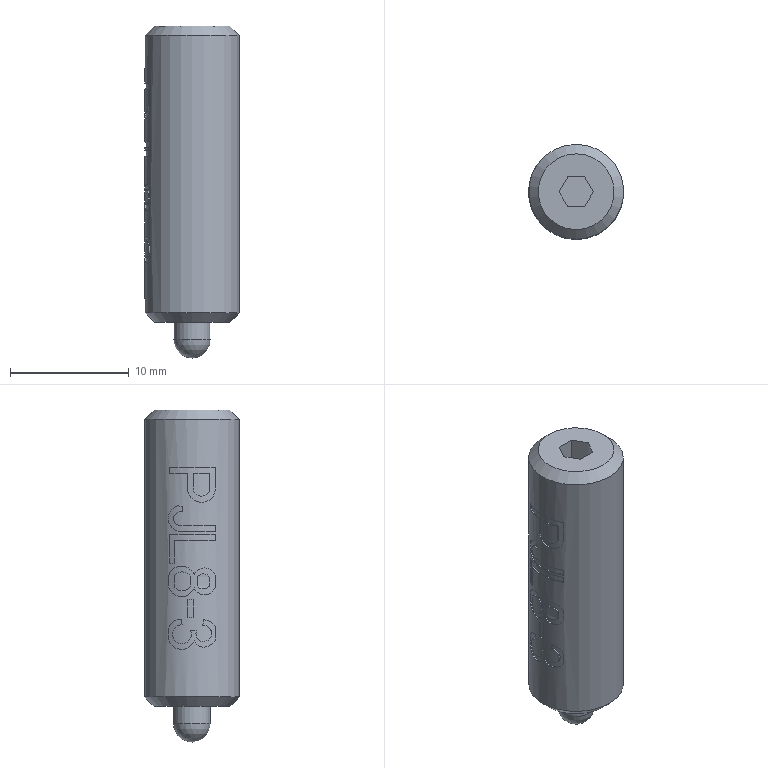Part | NX | features MI_PJL_0862 2 | 1 solid | 78 faces | box 8 x 8 x 28 mm | volume 1245 mm3 | plane 44 | cylinder 31 | cone 2 | sphere 1 | commonest cylinder face diameters 7.8 x6 8 x4 1.277 x2 1.595 x2 2.325 x2 1.168 x1